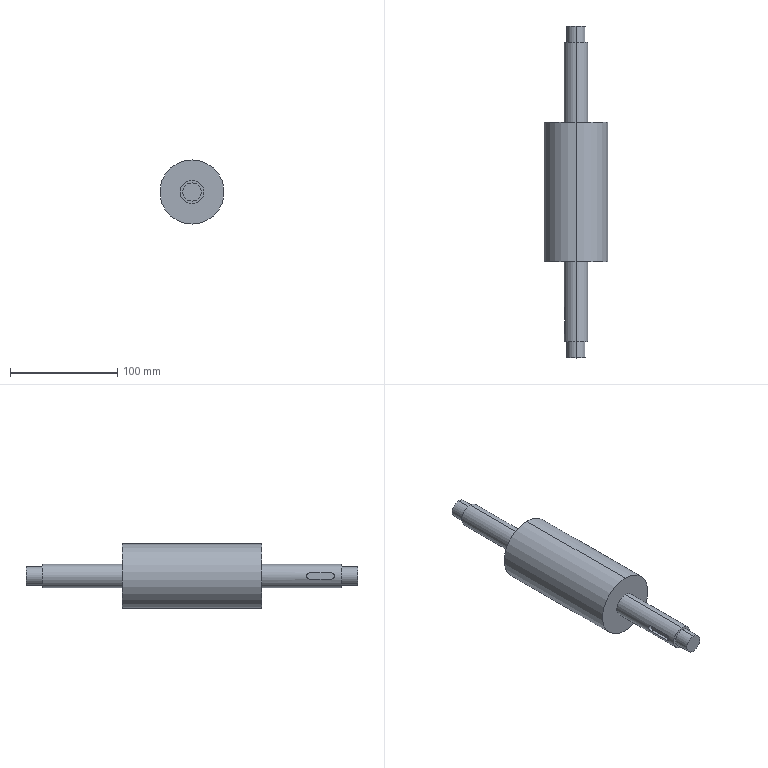Part | STEP file | A14-013 | 1 solid | 21 faces | box 60 x 310 x 60 mm | volume 430941 mm3 | cylinder 12 | plane 9 | commonest cylinder face diameters 17 x4 22 x4 6 x2 60 x2